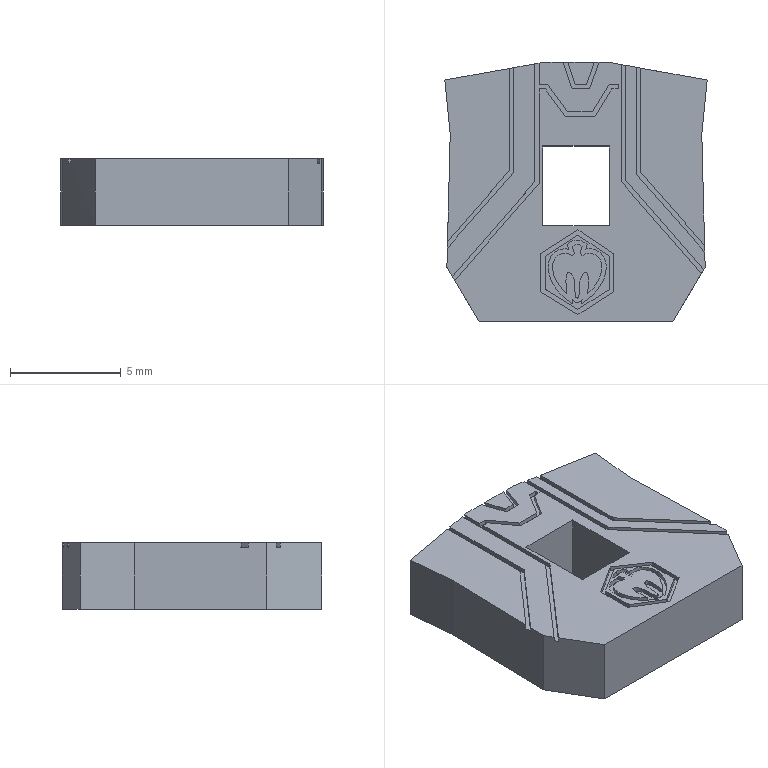Part | SolidWorks | features BaseBody 1 | 1 solid | 104 faces | box 11.849 x 11.702 x 3 mm | volume 350.145 mm3 | plane 74 | spline 30